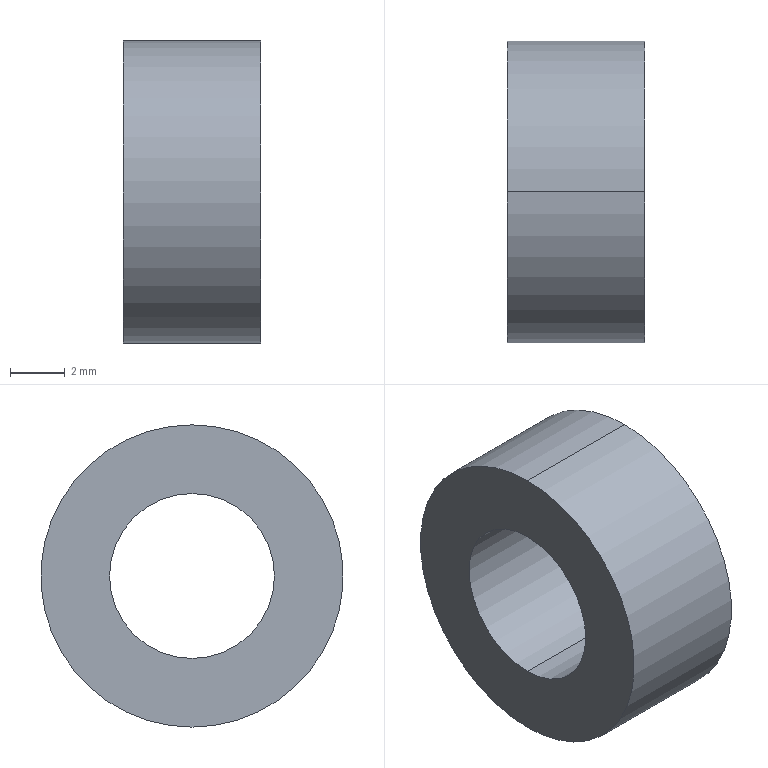Part | SolidWorks | features Extrusion 1 | 1 solid | 6 faces | box 5 x 11 x 11 mm | volume 333.794 mm3 | cylinder 4 | plane 2 | commonest cylinder face diameters 6 x2 11 x2
STEP:
#1=CARTESIAN_POINT('',(5.,0.,3.));
#2=VERTEX_POINT('',#1);
#3=CARTESIAN_POINT('',(5.,0.,-3.));
#4=VERTEX_POINT('',#3);
#5=CARTESIAN_POINT('',(5.,0.,0.));
#6=DIRECTION('',(1.,0.,0.));
#7=DIRECTION('',(0.,0.,-1.));
#8=AXIS2_PLACEMENT_3D('',#5,#6,#7);
#9=CIRCLE('',#8,3.);
#10=EDGE_CURVE('',#2,#4,#9,.T.);
#11=ORIENTED_EDGE('',*,*,#10,.T.);
#12=CARTESIAN_POINT('',(0.,0.,-3.));
#13=VERTEX_POINT('',#12);
#14=CARTESIAN_POINT('',(5.,0.,-3.));
#15=DIRECTION('',(-1.,0.,0.));
#16=VECTOR('',#15,1000.);
#17=LINE('',#14,#16);
#18=EDGE_CURVE('',#4,#13,#17,.T.);
#19=ORIENTED_EDGE('',*,*,#18,.T.);
#20=CARTESIAN_POINT('',(0.,0.,3.));
#21=VERTEX_POINT('',#20);
#22=CARTESIAN_POINT('',(0.,0.,0.));
#23=DIRECTION('',(1.,0.,0.));
#24=DIRECTION('',(0.,0.,-1.));
#25=AXIS2_PLACEMENT_3D('',#22,#23,#24);
#26=CIRCLE('',#25,3.);
#27=EDGE_CURVE('',#21,#13,#26,.T.);
#28=ORIENTED_EDGE('',*,*,#27,.F.);
#29=CARTESIAN_POINT('',(5.,0.,3.));
#30=DIRECTION('',(-1.,0.,0.));
#31=VECTOR('',#30,1000.);
#32=LINE('',#29,#31);
#33=EDGE_CURVE('',#2,#21,#32,.T.);
#34=ORIENTED_EDGE('',*,*,#33,.F.);
#35=EDGE_LOOP('',(#11,#19,#28,#34));
#36=FACE_OUTER_BOUND('',#35,.T.);
#37=CARTESIAN_POINT('',(5.,0.,0.));
#38=DIRECTION('',(-1.,0.,0.));
#39=DIRECTION('',(0.,0.,1.));
#40=AXIS2_PLACEMENT_3D('',#37,#38,#39);
#41=CYLINDRICAL_SURFACE('',#40,3.);
#42=ADVANCED_FACE('',(#36),#41,.F.);
#43=CARTESIAN_POINT('',(5.,0.,-5.5));
#44=VERTEX_POINT('',#43);
#45=CARTESIAN_POINT('',(5.,0.,5.5));
#46=VERTEX_POINT('',#45);
#47=CARTESIAN_POINT('',(5.,0.,0.));
#48=DIRECTION('',(1.,0.,0.));
#49=DIRECTION('',(0.,0.,-1.));
#50=AXIS2_PLACEMENT_3D('',#47,#48,#49);
#51=CIRCLE('',#50,5.5);
#52=EDGE_CURVE('',#44,#46,#51,.T.);
#53=ORIENTED_EDGE('',*,*,#52,.F.);
#54=CARTESIAN_POINT('',(0.,0.,-5.5));
#55=VERTEX_POINT('',#54);
#56=CARTESIAN_POINT('',(5.,0.,-5.5));
#57=DIRECTION('',(-1.,0.,0.));
#58=VECTOR('',#57,1000.);
#59=LINE('',#56,#58);
#60=EDGE_CURVE('',#44,#55,#59,.T.);
#61=ORIENTED_EDGE('',*,*,#60,.T.);
#62=CARTESIAN_POINT('',(0.,0.,5.5));
#63=VERTEX_POINT('',#62);
#64=CARTESIAN_POINT('',(0.,0.,0.));
#65=DIRECTION('',(1.,0.,0.));
#66=DIRECTION('',(0.,0.,-1.));
#67=AXIS2_PLACEMENT_3D('',#64,#65,#66);
#68=CIRCLE('',#67,5.5);
#69=EDGE_CURVE('',#55,#63,#68,.T.);
#70=ORIENTED_EDGE('',*,*,#69,.T.);
#71=CARTESIAN_POINT('',(5.,0.,5.5));
#72=DIRECTION('',(-1.,0.,0.));
#73=VECTOR('',#72,1000.);
#74=LINE('',#71,#73);
#75=EDGE_CURVE('',#46,#63,#74,.T.);
#76=ORIENTED_EDGE('',*,*,#75,.F.);
#77=EDGE_LOOP('',(#53,#61,#70,#76));
#78=FACE_OUTER_BOUND('',#77,.T.);
#79=CARTESIAN_POINT('',(5.,0.,0.));
#80=DIRECTION('',(-1.,0.,0.));
#81=DIRECTION('',(0.,0.,1.));
#82=AXIS2_PLACEMENT_3D('',#79,#80,#81);
#83=CYLINDRICAL_SURFACE('',#82,5.5);
#84=ADVANCED_FACE('',(#78),#83,.T.);
#85=CARTESIAN_POINT('',(5.,0.,0.));
#86=DIRECTION('',(1.,0.,0.));
#87=DIRECTION('',(0.,0.,-1.));
#88=AXIS2_PLACEMENT_3D('',#85,#86,#87);
#89=CIRCLE('',#88,5.5);
#90=EDGE_CURVE('',#46,#44,#89,.T.);
#91=ORIENTED_EDGE('',*,*,#90,.T.);
#92=ORIENTED_EDGE('',*,*,#52,.T.);
#93=EDGE_LOOP('',(#91,#92));
#94=FACE_OUTER_BOUND('',#93,.T.);
#95=ORIENTED_EDGE('',*,*,#10,.F.);
#96=CARTESIAN_POINT('',(5.,0.,0.));
#97=DIRECTION('',(1.,0.,0.));
#98=DIRECTION('',(0.,0.,-1.));
#99=AXIS2_PLACEMENT_3D('',#96,#97,#98);
#100=CIRCLE('',#99,3.);
#101=EDGE_CURVE('',#4,#2,#100,.T.);
#102=ORIENTED_EDGE('',*,*,#101,.F.);
#103=EDGE_LOOP('',(#95,#102));
#104=FACE_BOUND('',#103,.T.);
#105=CARTESIAN_POINT('',(5.,0.,0.));
#106=DIRECTION('',(1.,0.,0.));
#107=DIRECTION('',(0.,0.,-1.));
#108=AXIS2_PLACEMENT_3D('',#105,#106,#107);
#109=PLANE('',#108);
#110=ADVANCED_FACE('',(#94,#104),#109,.T.);
#111=CARTESIAN_POINT('',(0.,0.,0.));
#112=DIRECTION('',(1.,0.,0.));
#113=DIRECTION('',(0.,0.,-1.));
#114=AXIS2_PLACEMENT_3D('',#111,#112,#113);
#115=CIRCLE('',#114,5.5);
#116=EDGE_CURVE('',#63,#55,#115,.T.);
#117=ORIENTED_EDGE('',*,*,#116,.F.);
#118=ORIENTED_EDGE('',*,*,#69,.F.);
#119=EDGE_LOOP('',(#117,#118));
#120=FACE_OUTER_BOUND('',#119,.T.);
#121=ORIENTED_EDGE('',*,*,#27,.T.);
#122=CARTESIAN_POINT('',(0.,0.,0.));
#123=DIRECTION('',(1.,0.,0.));
#124=DIRECTION('',(0.,0.,-1.));
#125=AXIS2_PLACEMENT_3D('',#122,#123,#124);
#126=CIRCLE('',#125,3.);
#127=EDGE_CURVE('',#13,#21,#126,.T.);
#128=ORIENTED_EDGE('',*,*,#127,.T.);
#129=EDGE_LOOP('',(#121,#128));
#130=FACE_BOUND('',#129,.T.);
#131=CARTESIAN_POINT('',(0.,0.,0.));
#132=DIRECTION('',(1.,0.,0.));
#133=DIRECTION('',(0.,0.,-1.));
#134=AXIS2_PLACEMENT_3D('',#131,#132,#133);
#135=PLANE('',#134);
#136=ADVANCED_FACE('',(#120,#130),#135,.F.);
#137=ORIENTED_EDGE('',*,*,#60,.F.);
#138=ORIENTED_EDGE('',*,*,#90,.F.);
#139=ORIENTED_EDGE('',*,*,#75,.T.);
#140=ORIENTED_EDGE('',*,*,#116,.T.);
#141=EDGE_LOOP('',(#137,#138,#139,#140));
#142=FACE_OUTER_BOUND('',#141,.T.);
#143=CARTESIAN_POINT('',(5.,0.,0.));
#144=DIRECTION('',(-1.,0.,0.));
#145=DIRECTION('',(0.,0.,1.));
#146=AXIS2_PLACEMENT_3D('',#143,#144,#145);
#147=CYLINDRICAL_SURFACE('',#146,5.5);
#148=ADVANCED_FACE('',(#142),#147,.T.);
#149=ORIENTED_EDGE('',*,*,#18,.F.);
#150=ORIENTED_EDGE('',*,*,#101,.T.);
#151=ORIENTED_EDGE('',*,*,#33,.T.);
#152=ORIENTED_EDGE('',*,*,#127,.F.);
#153=EDGE_LOOP('',(#149,#150,#151,#152));
#154=FACE_OUTER_BOUND('',#153,.T.);
#155=CARTESIAN_POINT('',(5.,0.,0.));
#156=DIRECTION('',(-1.,0.,0.));
#157=DIRECTION('',(0.,0.,1.));
#158=AXIS2_PLACEMENT_3D('',#155,#156,#157);
#159=CYLINDRICAL_SURFACE('',#158,3.);
#160=ADVANCED_FACE('',(#154),#159,.F.);
#161=CLOSED_SHELL('',(#42,#84,#110,#136,#148,#160));
#162=MANIFOLD_SOLID_BREP('',#161);
#163=CARTESIAN_POINT('',(0.,0.,0.));
#164=DIRECTION('',(0.,0.,1.));
#165=DIRECTION('',(1.,0.,0.));
#166=AXIS2_PLACEMENT_3D('',#163,#164,#165);
#167=(LENGTH_UNIT()NAMED_UNIT(*)SI_UNIT(.MILLI.,.METRE.));
#168=UNCERTAINTY_MEASURE_WITH_UNIT(LENGTH_MEASURE(0.00001),#167,'','');
#169=(NAMED_UNIT(*)PLANE_ANGLE_UNIT()SI_UNIT($,.RADIAN.));
#170=(NAMED_UNIT(*)SI_UNIT($,.STERADIAN.)SOLID_ANGLE_UNIT());
#171=(GEOMETRIC_REPRESENTATION_CONTEXT(3)GLOBAL_UNCERTAINTY_ASSIGNED_CONTEXT((#168))GLOBAL_UNIT_ASSIGNED_CONTEXT((#167,#169,#170))REPRESENTATION_CONTEXT('',''));
#172=ADVANCED_BREP_SHAPE_REPRESENTATION('',(#162,#166),#171);